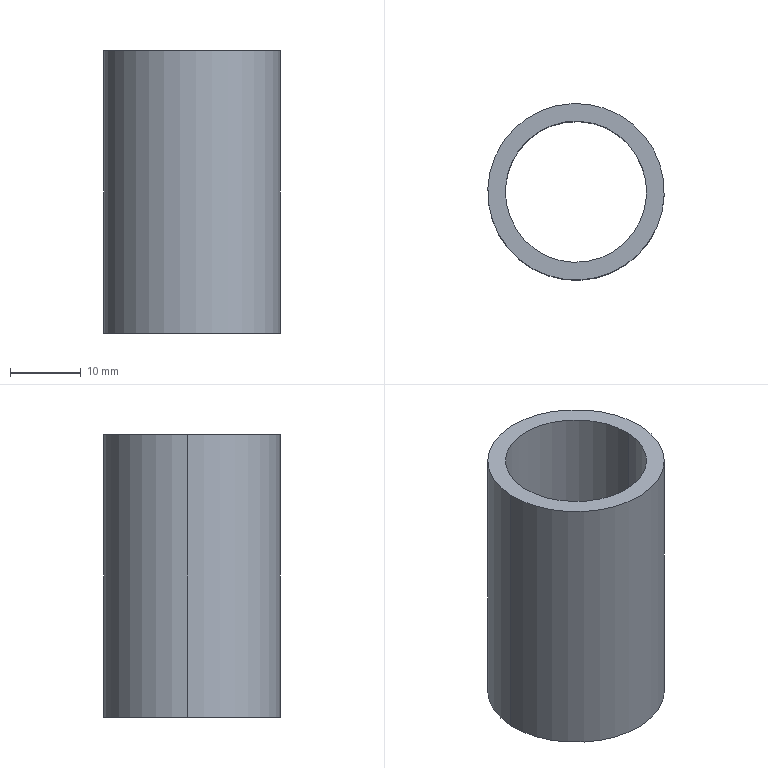Part | SolidWorks | features BaseBody 1 | 1 solid | 6 faces | box 25 x 25 x 40 mm | volume 7069 mm3 | cylinder 4 | plane 2 | commonest cylinder face diameters 20 x2 25 x2
STEP:
#1=CARTESIAN_POINT('',(-745.617,681.8,887.232));
#2=VERTEX_POINT('',#1);
#3=CARTESIAN_POINT('',(-720.645,680.621,887.232));
#4=VERTEX_POINT('',#3);
#5=CARTESIAN_POINT('',(-733.131,681.211,887.232));
#6=DIRECTION('',(0.,0.,-1.));
#7=DIRECTION('',(-0.9989,0.04718,0.));
#8=AXIS2_PLACEMENT_3D('',#5,#6,#7);
#9=CIRCLE('',#8,12.5);
#10=EDGE_CURVE('',#2,#4,#9,.T.);
#11=ORIENTED_EDGE('',*,*,#10,.F.);
#12=CARTESIAN_POINT('',(-733.131,681.211,887.232));
#13=DIRECTION('',(0.,0.,-1.));
#14=DIRECTION('',(0.9989,-0.04718,0.));
#15=AXIS2_PLACEMENT_3D('',#12,#13,#14);
#16=CIRCLE('',#15,12.5);
#17=EDGE_CURVE('',#4,#2,#16,.T.);
#18=ORIENTED_EDGE('',*,*,#17,.F.);
#19=EDGE_LOOP('',(#11,#18));
#20=FACE_OUTER_BOUND('',#19,.T.);
#21=CARTESIAN_POINT('',(-723.142,680.739,887.232));
#22=VERTEX_POINT('',#21);
#23=CARTESIAN_POINT('',(-743.12,681.682,887.232));
#24=VERTEX_POINT('',#23);
#25=CARTESIAN_POINT('',(-733.131,681.211,887.232));
#26=DIRECTION('',(0.,0.,1.));
#27=DIRECTION('',(0.9989,-0.04718,0.));
#28=AXIS2_PLACEMENT_3D('',#25,#26,#27);
#29=CIRCLE('',#28,10.);
#30=EDGE_CURVE('',#22,#24,#29,.T.);
#31=ORIENTED_EDGE('',*,*,#30,.F.);
#32=CARTESIAN_POINT('',(-733.131,681.211,887.232));
#33=DIRECTION('',(0.,0.,1.));
#34=DIRECTION('',(-0.9989,0.04718,0.));
#35=AXIS2_PLACEMENT_3D('',#32,#33,#34);
#36=CIRCLE('',#35,10.);
#37=EDGE_CURVE('',#24,#22,#36,.T.);
#38=ORIENTED_EDGE('',*,*,#37,.F.);
#39=EDGE_LOOP('',(#31,#38));
#40=FACE_BOUND('',#39,.T.);
#41=CARTESIAN_POINT('',(-733.131,681.211,887.232));
#42=DIRECTION('',(0.,0.,1.));
#43=DIRECTION('',(0.9989,-0.04718,0.));
#44=AXIS2_PLACEMENT_3D('',#41,#42,#43);
#45=PLANE('',#44);
#46=ADVANCED_FACE('',(#20,#40),#45,.T.);
#47=CARTESIAN_POINT('',(-745.617,681.8,847.232));
#48=VERTEX_POINT('',#47);
#49=CARTESIAN_POINT('',(-720.645,680.621,847.232));
#50=VERTEX_POINT('',#49);
#51=CARTESIAN_POINT('',(-733.131,681.211,847.232));
#52=DIRECTION('',(0.,0.,1.));
#53=DIRECTION('',(-0.9989,0.04718,0.));
#54=AXIS2_PLACEMENT_3D('',#51,#52,#53);
#55=CIRCLE('',#54,12.5);
#56=EDGE_CURVE('',#48,#50,#55,.T.);
#57=ORIENTED_EDGE('',*,*,#56,.T.);
#58=CARTESIAN_POINT('',(-720.645,680.621,847.232));
#59=DIRECTION('',(0.,0.,1.));
#60=VECTOR('',#59,1000.);
#61=LINE('',#58,#60);
#62=EDGE_CURVE('',#50,#4,#61,.T.);
#63=ORIENTED_EDGE('',*,*,#62,.T.);
#64=ORIENTED_EDGE('',*,*,#17,.T.);
#65=CARTESIAN_POINT('',(-745.617,681.8,887.232));
#66=DIRECTION('',(0.,0.,-1.));
#67=VECTOR('',#66,1000.);
#68=LINE('',#65,#67);
#69=EDGE_CURVE('',#2,#48,#68,.T.);
#70=ORIENTED_EDGE('',*,*,#69,.T.);
#71=EDGE_LOOP('',(#57,#63,#64,#70));
#72=FACE_OUTER_BOUND('',#71,.T.);
#73=CARTESIAN_POINT('',(-733.131,681.211,887.232));
#74=DIRECTION('',(0.,0.,-1.));
#75=DIRECTION('',(-0.9989,0.04718,0.));
#76=AXIS2_PLACEMENT_3D('',#73,#74,#75);
#77=CYLINDRICAL_SURFACE('',#76,12.5);
#78=ADVANCED_FACE('',(#72),#77,.T.);
#79=ORIENTED_EDGE('',*,*,#62,.F.);
#80=CARTESIAN_POINT('',(-733.131,681.211,847.232));
#81=DIRECTION('',(0.,0.,1.));
#82=DIRECTION('',(0.9989,-0.04718,0.));
#83=AXIS2_PLACEMENT_3D('',#80,#81,#82);
#84=CIRCLE('',#83,12.5);
#85=EDGE_CURVE('',#50,#48,#84,.T.);
#86=ORIENTED_EDGE('',*,*,#85,.T.);
#87=ORIENTED_EDGE('',*,*,#69,.F.);
#88=ORIENTED_EDGE('',*,*,#10,.T.);
#89=EDGE_LOOP('',(#79,#86,#87,#88));
#90=FACE_OUTER_BOUND('',#89,.T.);
#91=CARTESIAN_POINT('',(-733.131,681.211,887.232));
#92=DIRECTION('',(0.,0.,-1.));
#93=DIRECTION('',(-0.9989,0.04718,0.));
#94=AXIS2_PLACEMENT_3D('',#91,#92,#93);
#95=CYLINDRICAL_SURFACE('',#94,12.5);
#96=ADVANCED_FACE('',(#90),#95,.T.);
#97=ORIENTED_EDGE('',*,*,#85,.F.);
#98=ORIENTED_EDGE('',*,*,#56,.F.);
#99=EDGE_LOOP('',(#97,#98));
#100=FACE_OUTER_BOUND('',#99,.T.);
#101=CARTESIAN_POINT('',(-743.12,681.682,847.232));
#102=VERTEX_POINT('',#101);
#103=CARTESIAN_POINT('',(-723.142,680.739,847.232));
#104=VERTEX_POINT('',#103);
#105=CARTESIAN_POINT('',(-733.131,681.211,847.232));
#106=DIRECTION('',(0.,0.,-1.));
#107=DIRECTION('',(-0.9989,0.04718,0.));
#108=AXIS2_PLACEMENT_3D('',#105,#106,#107);
#109=CIRCLE('',#108,10.);
#110=EDGE_CURVE('',#102,#104,#109,.T.);
#111=ORIENTED_EDGE('',*,*,#110,.F.);
#112=CARTESIAN_POINT('',(-733.131,681.211,847.232));
#113=DIRECTION('',(0.,0.,-1.));
#114=DIRECTION('',(0.9989,-0.04718,0.));
#115=AXIS2_PLACEMENT_3D('',#112,#113,#114);
#116=CIRCLE('',#115,10.);
#117=EDGE_CURVE('',#104,#102,#116,.T.);
#118=ORIENTED_EDGE('',*,*,#117,.F.);
#119=EDGE_LOOP('',(#111,#118));
#120=FACE_BOUND('',#119,.T.);
#121=CARTESIAN_POINT('',(-733.131,681.211,847.232));
#122=DIRECTION('',(0.,0.,1.));
#123=DIRECTION('',(0.9989,-0.04718,0.));
#124=AXIS2_PLACEMENT_3D('',#121,#122,#123);
#125=PLANE('',#124);
#126=ADVANCED_FACE('',(#100,#120),#125,.F.);
#127=CARTESIAN_POINT('',(-723.142,680.739,887.232));
#128=DIRECTION('',(0.,0.,-1.));
#129=VECTOR('',#128,1000.);
#130=LINE('',#127,#129);
#131=EDGE_CURVE('',#22,#104,#130,.T.);
#132=ORIENTED_EDGE('',*,*,#131,.T.);
#133=ORIENTED_EDGE('',*,*,#117,.T.);
#134=CARTESIAN_POINT('',(-743.12,681.682,847.232));
#135=DIRECTION('',(0.,0.,1.));
#136=VECTOR('',#135,1000.);
#137=LINE('',#134,#136);
#138=EDGE_CURVE('',#102,#24,#137,.T.);
#139=ORIENTED_EDGE('',*,*,#138,.T.);
#140=ORIENTED_EDGE('',*,*,#37,.T.);
#141=EDGE_LOOP('',(#132,#133,#139,#140));
#142=FACE_OUTER_BOUND('',#141,.T.);
#143=CARTESIAN_POINT('',(-733.131,681.211,887.232));
#144=DIRECTION('',(0.,0.,-1.));
#145=DIRECTION('',(-0.9989,0.04718,0.));
#146=AXIS2_PLACEMENT_3D('',#143,#144,#145);
#147=CYLINDRICAL_SURFACE('',#146,10.);
#148=ADVANCED_FACE('',(#142),#147,.F.);
#149=ORIENTED_EDGE('',*,*,#110,.T.);
#150=ORIENTED_EDGE('',*,*,#131,.F.);
#151=ORIENTED_EDGE('',*,*,#30,.T.);
#152=ORIENTED_EDGE('',*,*,#138,.F.);
#153=EDGE_LOOP('',(#149,#150,#151,#152));
#154=FACE_OUTER_BOUND('',#153,.T.);
#155=CARTESIAN_POINT('',(-733.131,681.211,887.232));
#156=DIRECTION('',(0.,0.,-1.));
#157=DIRECTION('',(-0.9989,0.04718,0.));
#158=AXIS2_PLACEMENT_3D('',#155,#156,#157);
#159=CYLINDRICAL_SURFACE('',#158,10.);
#160=ADVANCED_FACE('',(#154),#159,.F.);
#161=CLOSED_SHELL('',(#46,#78,#96,#126,#148,#160));
#162=MANIFOLD_SOLID_BREP('',#161);
#163=CARTESIAN_POINT('',(0.,0.,0.));
#164=DIRECTION('',(0.,0.,1.));
#165=DIRECTION('',(1.,0.,0.));
#166=AXIS2_PLACEMENT_3D('',#163,#164,#165);
#167=(LENGTH_UNIT()NAMED_UNIT(*)SI_UNIT(.MILLI.,.METRE.));
#168=UNCERTAINTY_MEASURE_WITH_UNIT(LENGTH_MEASURE(0.00001),#167,'','');
#169=(NAMED_UNIT(*)PLANE_ANGLE_UNIT()SI_UNIT($,.RADIAN.));
#170=(NAMED_UNIT(*)SI_UNIT($,.STERADIAN.)SOLID_ANGLE_UNIT());
#171=(GEOMETRIC_REPRESENTATION_CONTEXT(3)GLOBAL_UNCERTAINTY_ASSIGNED_CONTEXT((#168))GLOBAL_UNIT_ASSIGNED_CONTEXT((#167,#169,#170))REPRESENTATION_CONTEXT('',''));
#172=ADVANCED_BREP_SHAPE_REPRESENTATION('',(#162,#166),#171);